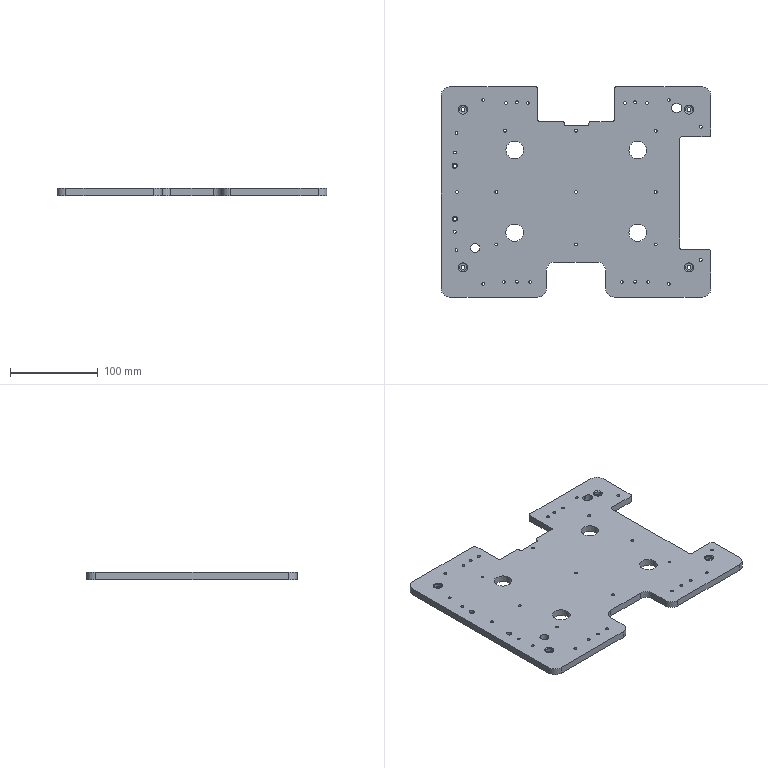Part | 1 solid | 110 faces | box 308 x 240 x 8 mm | volume 488350 mm3 | cylinder 71 | plane 32 | cone 7 | commonest cylinder face diameters 3.3 x32 4 x14 20 x12 4.5 x4 8.5 x4 6.05 x2